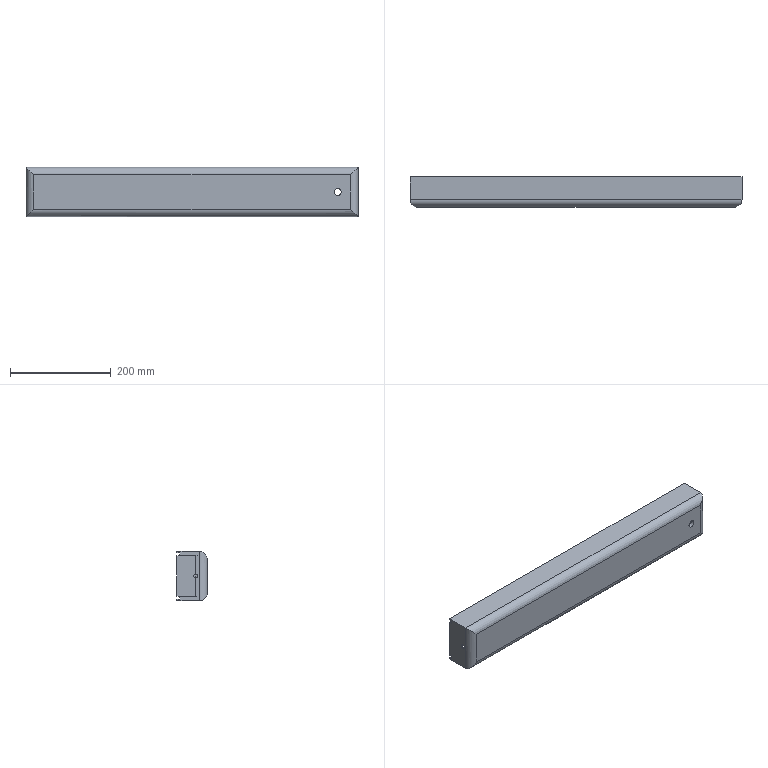Part | SolidWorks | features BaseBody 1 | 1 solid | 34 faces | box 660 x 60.3 x 97.82 mm | volume 1057763 mm3 | plane 22 | cylinder 12 | commonest cylinder face diameters 30 x8 8 x2 14 x2
STEP:
#1=CARTESIAN_POINT('',(-747.81,92.16,59.05));
#2=VERTEX_POINT('',#1);
#3=CARTESIAN_POINT('',(-750.,92.16,59.05));
#4=VERTEX_POINT('',#3);
#5=CARTESIAN_POINT('',(-747.81,92.16,59.05));
#6=DIRECTION('',(-1.,0.,0.));
#7=VECTOR('',#6,1000.);
#8=LINE('',#5,#7);
#9=EDGE_CURVE('',#2,#4,#8,.T.);
#10=ORIENTED_EDGE('',*,*,#9,.F.);
#11=CARTESIAN_POINT('',(-747.81,92.16,-21.25));
#12=VERTEX_POINT('',#11);
#13=CARTESIAN_POINT('',(-747.81,92.16,-21.25));
#14=DIRECTION('',(0.,0.,1.));
#15=VECTOR('',#14,1000.);
#16=LINE('',#13,#15);
#17=EDGE_CURVE('',#12,#2,#16,.T.);
#18=ORIENTED_EDGE('',*,*,#17,.F.);
#19=CARTESIAN_POINT('',(-750.,92.16,-21.25));
#20=VERTEX_POINT('',#19);
#21=CARTESIAN_POINT('',(-750.,92.16,-21.25));
#22=DIRECTION('',(1.,0.,0.));
#23=VECTOR('',#22,1000.);
#24=LINE('',#21,#23);
#25=EDGE_CURVE('',#20,#12,#24,.T.);
#26=ORIENTED_EDGE('',*,*,#25,.F.);
#27=CARTESIAN_POINT('',(-750.,92.16,59.05));
#28=DIRECTION('',(0.,0.,-1.));
#29=VECTOR('',#28,1000.);
#30=LINE('',#27,#29);
#31=EDGE_CURVE('',#4,#20,#30,.T.);
#32=ORIENTED_EDGE('',*,*,#31,.F.);
#33=EDGE_LOOP('',(#10,#18,#26,#32));
#34=FACE_OUTER_BOUND('',#33,.T.);
#35=CARTESIAN_POINT('',(-1290.2,92.16,18.9));
#36=DIRECTION('',(0.,1.,0.));
#37=DIRECTION('',(1.,0.,0.));
#38=AXIS2_PLACEMENT_3D('',#35,#36,#37);
#39=PLANE('',#38);
#40=ADVANCED_FACE('',(#34),#39,.T.);
#41=CARTESIAN_POINT('',(-750.,86.32,-21.25));
#42=VERTEX_POINT('',#41);
#43=CARTESIAN_POINT('',(-747.81,86.32,-21.25));
#44=VERTEX_POINT('',#43);
#45=CARTESIAN_POINT('',(-750.,86.32,-21.25));
#46=DIRECTION('',(1.,0.,0.));
#47=VECTOR('',#46,1000.);
#48=LINE('',#45,#47);
#49=EDGE_CURVE('',#42,#44,#48,.T.);
#50=ORIENTED_EDGE('',*,*,#49,.F.);
#51=CARTESIAN_POINT('',(-750.,92.16,-21.25));
#52=DIRECTION('',(0.,-1.,0.));
#53=VECTOR('',#52,1000.);
#54=LINE('',#51,#53);
#55=EDGE_CURVE('',#20,#42,#54,.T.);
#56=ORIENTED_EDGE('',*,*,#55,.F.);
#57=ORIENTED_EDGE('',*,*,#25,.T.);
#58=CARTESIAN_POINT('',(-747.81,86.32,-21.25));
#59=DIRECTION('',(0.,1.,0.));
#60=VECTOR('',#59,1000.);
#61=LINE('',#58,#60);
#62=EDGE_CURVE('',#44,#12,#61,.T.);
#63=ORIENTED_EDGE('',*,*,#62,.F.);
#64=EDGE_LOOP('',(#50,#56,#57,#63));
#65=FACE_OUTER_BOUND('',#64,.T.);
#66=CARTESIAN_POINT('',(-750.,92.16,-21.25));
#67=DIRECTION('',(0.,0.,-1.));
#68=DIRECTION('',(0.,-1.,0.));
#69=AXIS2_PLACEMENT_3D('',#66,#67,#68);
#70=PLANE('',#69);
#71=ADVANCED_FACE('',(#65),#70,.T.);
#72=CARTESIAN_POINT('',(-747.81,86.32,59.05));
#73=VERTEX_POINT('',#72);
#74=CARTESIAN_POINT('',(-750.,86.32,59.05));
#75=VERTEX_POINT('',#74);
#76=CARTESIAN_POINT('',(-747.81,86.32,59.05));
#77=DIRECTION('',(-1.,0.,0.));
#78=VECTOR('',#77,1000.);
#79=LINE('',#76,#78);
#80=EDGE_CURVE('',#73,#75,#79,.T.);
#81=ORIENTED_EDGE('',*,*,#80,.F.);
#82=CARTESIAN_POINT('',(-747.81,92.16,59.05));
#83=DIRECTION('',(0.,-1.,0.));
#84=VECTOR('',#83,1000.);
#85=LINE('',#82,#84);
#86=EDGE_CURVE('',#2,#73,#85,.T.);
#87=ORIENTED_EDGE('',*,*,#86,.F.);
#88=ORIENTED_EDGE('',*,*,#9,.T.);
#89=CARTESIAN_POINT('',(-750.,86.32,59.05));
#90=DIRECTION('',(0.,1.,0.));
#91=VECTOR('',#90,1000.);
#92=LINE('',#89,#91);
#93=EDGE_CURVE('',#75,#4,#92,.T.);
#94=ORIENTED_EDGE('',*,*,#93,.F.);
#95=EDGE_LOOP('',(#81,#87,#88,#94));
#96=FACE_OUTER_BOUND('',#95,.T.);
#97=CARTESIAN_POINT('',(-750.,92.16,59.05));
#98=DIRECTION('',(0.,0.,1.));
#99=DIRECTION('',(1.,0.,0.));
#100=AXIS2_PLACEMENT_3D('',#97,#98,#99);
#101=PLANE('',#100);
#102=ADVANCED_FACE('',(#96),#101,.T.);
#103=CARTESIAN_POINT('',(-750.,92.16,-30.01));
#104=VERTEX_POINT('',#103);
#105=CARTESIAN_POINT('',(-90.,92.16,-30.01));
#106=VERTEX_POINT('',#105);
#107=CARTESIAN_POINT('',(-750.,92.16,-30.01));
#108=DIRECTION('',(1.,0.,0.));
#109=VECTOR('',#108,1000.);
#110=LINE('',#107,#109);
#111=EDGE_CURVE('',#104,#106,#110,.T.);
#112=ORIENTED_EDGE('',*,*,#111,.F.);
#113=CARTESIAN_POINT('',(-750.,92.16,-27.09));
#114=VERTEX_POINT('',#113);
#115=CARTESIAN_POINT('',(-750.,92.16,-27.09));
#116=DIRECTION('',(0.,0.,-1.));
#117=VECTOR('',#116,1000.);
#118=LINE('',#115,#117);
#119=EDGE_CURVE('',#114,#104,#118,.T.);
#120=ORIENTED_EDGE('',*,*,#119,.F.);
#121=CARTESIAN_POINT('',(-90.,92.16,-27.09));
#122=VERTEX_POINT('',#121);
#123=CARTESIAN_POINT('',(-90.,92.16,-27.09));
#124=DIRECTION('',(-1.,0.,0.));
#125=VECTOR('',#124,1000.);
#126=LINE('',#123,#125);
#127=EDGE_CURVE('',#122,#114,#126,.T.);
#128=ORIENTED_EDGE('',*,*,#127,.F.);
#129=CARTESIAN_POINT('',(-90.,92.16,-30.01));
#130=DIRECTION('',(0.,0.,1.));
#131=VECTOR('',#130,1000.);
#132=LINE('',#129,#131);
#133=EDGE_CURVE('',#106,#122,#132,.T.);
#134=ORIENTED_EDGE('',*,*,#133,.F.);
#135=EDGE_LOOP('',(#112,#120,#128,#134));
#136=FACE_OUTER_BOUND('',#135,.T.);
#137=CARTESIAN_POINT('',(-202.5,92.16,18.9));
#138=DIRECTION('',(0.,1.,0.));
#139=DIRECTION('',(1.,0.,0.));
#140=AXIS2_PLACEMENT_3D('',#137,#138,#139);
#141=PLANE('',#140);
#142=ADVANCED_FACE('',(#136),#141,.T.);
#143=ORIENTED_EDGE('',*,*,#127,.T.);
#144=CARTESIAN_POINT('',(-750.,86.32,-27.09));
#145=VERTEX_POINT('',#144);
#146=CARTESIAN_POINT('',(-750.,86.32,-27.09));
#147=DIRECTION('',(0.,1.,0.));
#148=VECTOR('',#147,1000.);
#149=LINE('',#146,#148);
#150=EDGE_CURVE('',#145,#114,#149,.T.);
#151=ORIENTED_EDGE('',*,*,#150,.F.);
#152=CARTESIAN_POINT('',(-90.,86.32,-27.09));
#153=VERTEX_POINT('',#152);
#154=CARTESIAN_POINT('',(-90.,86.32,-27.09));
#155=DIRECTION('',(-1.,0.,0.));
#156=VECTOR('',#155,1000.);
#157=LINE('',#154,#156);
#158=EDGE_CURVE('',#153,#145,#157,.T.);
#159=ORIENTED_EDGE('',*,*,#158,.F.);
#160=CARTESIAN_POINT('',(-90.,92.16,-27.09));
#161=DIRECTION('',(0.,-1.,0.));
#162=VECTOR('',#161,1000.);
#163=LINE('',#160,#162);
#164=EDGE_CURVE('',#122,#153,#163,.T.);
#165=ORIENTED_EDGE('',*,*,#164,.F.);
#166=EDGE_LOOP('',(#143,#151,#159,#165));
#167=FACE_OUTER_BOUND('',#166,.T.);
#168=CARTESIAN_POINT('',(-750.,92.16,-27.09));
#169=DIRECTION('',(0.,0.,1.));
#170=DIRECTION('',(1.,0.,0.));
#171=AXIS2_PLACEMENT_3D('',#168,#169,#170);
#172=PLANE('',#171);
#173=ADVANCED_FACE('',(#167),#172,.T.);
#174=ORIENTED_EDGE('',*,*,#158,.T.);
#175=CARTESIAN_POINT('',(-750.,86.32,-21.25));
#176=DIRECTION('',(0.,0.,-1.));
#177=VECTOR('',#176,1000.);
#178=LINE('',#175,#177);
#179=EDGE_CURVE('',#42,#145,#178,.T.);
#180=ORIENTED_EDGE('',*,*,#179,.F.);
#181=ORIENTED_EDGE('',*,*,#49,.T.);
#182=CARTESIAN_POINT('',(-93.,86.32,-21.25));
#183=VERTEX_POINT('',#182);
#184=CARTESIAN_POINT('',(-93.,86.32,-21.25));
#185=DIRECTION('',(-1.,0.,0.));
#186=VECTOR('',#185,1000.);
#187=LINE('',#184,#186);
#188=EDGE_CURVE('',#183,#44,#187,.T.);
#189=ORIENTED_EDGE('',*,*,#188,.F.);
#190=CARTESIAN_POINT('',(-90.,86.32,-21.25));
#191=VERTEX_POINT('',#190);
#192=CARTESIAN_POINT('',(-90.,86.32,-21.25));
#193=DIRECTION('',(-1.,0.,0.));
#194=VECTOR('',#193,1000.);
#195=LINE('',#192,#194);
#196=EDGE_CURVE('',#191,#183,#195,.T.);
#197=ORIENTED_EDGE('',*,*,#196,.F.);
#198=CARTESIAN_POINT('',(-90.,86.32,-27.09));
#199=DIRECTION('',(0.,0.,1.));
#200=VECTOR('',#199,1000.);
#201=LINE('',#198,#200);
#202=EDGE_CURVE('',#153,#191,#201,.T.);
#203=ORIENTED_EDGE('',*,*,#202,.F.);
#204=EDGE_LOOP('',(#174,#180,#181,#189,#197,#203));
#205=FACE_OUTER_BOUND('',#204,.T.);
#206=CARTESIAN_POINT('',(-750.,86.32,64.89));
#207=DIRECTION('',(0.,1.,0.));
#208=DIRECTION('',(1.,0.,0.));
#209=AXIS2_PLACEMENT_3D('',#206,#207,#208);
#210=PLANE('',#209);
#211=ADVANCED_FACE('',(#205),#210,.T.);
#212=CARTESIAN_POINT('',(-747.81,54.16,-21.25));
#213=VERTEX_POINT('',#212);
#214=CARTESIAN_POINT('',(-747.81,54.16,-21.25));
#215=DIRECTION('',(0.,1.,0.));
#216=VECTOR('',#215,1000.);
#217=LINE('',#214,#216);
#218=EDGE_CURVE('',#213,#44,#217,.T.);
#219=ORIENTED_EDGE('',*,*,#218,.F.);
#220=CARTESIAN_POINT('',(-93.,54.16,-21.25));
#221=VERTEX_POINT('',#220);
#222=CARTESIAN_POINT('',(-93.,54.16,-21.25));
#223=DIRECTION('',(-1.,0.,0.));
#224=VECTOR('',#223,1000.);
#225=LINE('',#222,#224);
#226=EDGE_CURVE('',#221,#213,#225,.T.);
#227=ORIENTED_EDGE('',*,*,#226,.F.);
#228=CARTESIAN_POINT('',(-93.,86.32,-21.25));
#229=DIRECTION('',(0.,-1.,0.));
#230=VECTOR('',#229,1000.);
#231=LINE('',#228,#230);
#232=EDGE_CURVE('',#183,#221,#231,.T.);
#233=ORIENTED_EDGE('',*,*,#232,.F.);
#234=ORIENTED_EDGE('',*,*,#188,.T.);
#235=EDGE_LOOP('',(#219,#227,#233,#234));
#236=FACE_OUTER_BOUND('',#235,.T.);
#237=CARTESIAN_POINT('',(-742.7,19.16,-21.25));
#238=DIRECTION('',(0.,0.,1.));
#239=DIRECTION('',(1.,0.,0.));
#240=AXIS2_PLACEMENT_3D('',#237,#238,#239);
#241=PLANE('',#240);
#242=ADVANCED_FACE('',(#236),#241,.T.);
#243=CARTESIAN_POINT('',(-93.,86.32,59.05));
#244=VERTEX_POINT('',#243);
#245=CARTESIAN_POINT('',(-747.81,86.32,59.05));
#246=DIRECTION('',(1.,0.,0.));
#247=VECTOR('',#246,1000.);
#248=LINE('',#245,#247);
#249=EDGE_CURVE('',#73,#244,#248,.T.);
#250=ORIENTED_EDGE('',*,*,#249,.F.);
#251=ORIENTED_EDGE('',*,*,#80,.T.);
#252=CARTESIAN_POINT('',(-750.,86.32,64.89));
#253=VERTEX_POINT('',#252);
#254=CARTESIAN_POINT('',(-750.,86.32,64.89));
#255=DIRECTION('',(0.,0.,-1.));
#256=VECTOR('',#255,1000.);
#257=LINE('',#254,#256);
#258=EDGE_CURVE('',#253,#75,#257,.T.);
#259=ORIENTED_EDGE('',*,*,#258,.F.);
#260=CARTESIAN_POINT('',(-90.,86.32,64.89));
#261=VERTEX_POINT('',#260);
#262=CARTESIAN_POINT('',(-90.,86.32,64.89));
#263=DIRECTION('',(-1.,0.,0.));
#264=VECTOR('',#263,1000.);
#265=LINE('',#262,#264);
#266=EDGE_CURVE('',#261,#253,#265,.T.);
#267=ORIENTED_EDGE('',*,*,#266,.F.);
#268=CARTESIAN_POINT('',(-90.,86.32,59.05));
#269=VERTEX_POINT('',#268);
#270=CARTESIAN_POINT('',(-90.,86.32,59.05));
#271=DIRECTION('',(0.,0.,1.));
#272=VECTOR('',#271,1000.);
#273=LINE('',#270,#272);
#274=EDGE_CURVE('',#269,#261,#273,.T.);
#275=ORIENTED_EDGE('',*,*,#274,.F.);
#276=CARTESIAN_POINT('',(-93.,86.32,59.05));
#277=DIRECTION('',(1.,0.,0.));
#278=VECTOR('',#277,1000.);
#279=LINE('',#276,#278);
#280=EDGE_CURVE('',#244,#269,#279,.T.);
#281=ORIENTED_EDGE('',*,*,#280,.F.);
#282=EDGE_LOOP('',(#250,#251,#259,#267,#275,#281));
#283=FACE_OUTER_BOUND('',#282,.T.);
#284=CARTESIAN_POINT('',(-750.,86.32,64.89));
#285=DIRECTION('',(0.,1.,0.));
#286=DIRECTION('',(1.,0.,0.));
#287=AXIS2_PLACEMENT_3D('',#284,#285,#286);
#288=PLANE('',#287);
#289=ADVANCED_FACE('',(#283),#288,.T.);
#290=ORIENTED_EDGE('',*,*,#266,.T.);
#291=CARTESIAN_POINT('',(-750.,92.16,64.89));
#292=VERTEX_POINT('',#291);
#293=CARTESIAN_POINT('',(-750.,92.16,64.89));
#294=DIRECTION('',(0.,-1.,0.));
#295=VECTOR('',#294,1000.);
#296=LINE('',#293,#295);
#297=EDGE_CURVE('',#292,#253,#296,.T.);
#298=ORIENTED_EDGE('',*,*,#297,.F.);
#299=CARTESIAN_POINT('',(-90.,92.16,64.89));
#300=VERTEX_POINT('',#299);
#301=CARTESIAN_POINT('',(-90.,92.16,64.89));
#302=DIRECTION('',(-1.,0.,0.));
#303=VECTOR('',#302,1000.);
#304=LINE('',#301,#303);
#305=EDGE_CURVE('',#300,#292,#304,.T.);
#306=ORIENTED_EDGE('',*,*,#305,.F.);
#307=CARTESIAN_POINT('',(-90.,86.32,64.89));
#308=DIRECTION('',(0.,1.,0.));
#309=VECTOR('',#308,1000.);
#310=LINE('',#307,#309);
#311=EDGE_CURVE('',#261,#300,#310,.T.);
#312=ORIENTED_EDGE('',*,*,#311,.F.);
#313=EDGE_LOOP('',(#290,#298,#306,#312));
#314=FACE_OUTER_BOUND('',#313,.T.);
#315=CARTESIAN_POINT('',(-750.,92.16,64.89));
#316=DIRECTION('',(0.,0.,-1.));
#317=DIRECTION('',(0.,-1.,0.));
#318=AXIS2_PLACEMENT_3D('',#315,#316,#317);
#319=PLANE('',#318);
#320=ADVANCED_FACE('',(#314),#319,.T.);
#321=ORIENTED_EDGE('',*,*,#305,.T.);
#322=CARTESIAN_POINT('',(-750.,92.16,67.81));
#323=VERTEX_POINT('',#322);
#324=CARTESIAN_POINT('',(-750.,92.16,67.81));
#325=DIRECTION('',(0.,0.,-1.));
#326=VECTOR('',#325,1000.);
#327=LINE('',#324,#326);
#328=EDGE_CURVE('',#323,#292,#327,.T.);
#329=ORIENTED_EDGE('',*,*,#328,.F.);
#330=CARTESIAN_POINT('',(-90.,92.16,67.81));
#331=VERTEX_POINT('',#330);
#332=CARTESIAN_POINT('',(-90.,92.16,67.81));
#333=DIRECTION('',(-1.,0.,0.));
#334=VECTOR('',#333,1000.);
#335=LINE('',#332,#334);
#336=EDGE_CURVE('',#331,#323,#335,.T.);
#337=ORIENTED_EDGE('',*,*,#336,.F.);
#338=CARTESIAN_POINT('',(-90.,92.16,64.89));
#339=DIRECTION('',(0.,0.,1.));
#340=VECTOR('',#339,1000.);
#341=LINE('',#338,#340);
#342=EDGE_CURVE('',#300,#331,#341,.T.);
#343=ORIENTED_EDGE('',*,*,#342,.F.);
#344=EDGE_LOOP('',(#321,#329,#337,#343));
#345=FACE_OUTER_BOUND('',#344,.T.);
#346=CARTESIAN_POINT('',(-202.5,92.16,18.9));
#347=DIRECTION('',(0.,1.,0.));
#348=DIRECTION('',(1.,0.,0.));
#349=AXIS2_PLACEMENT_3D('',#346,#347,#348);
#350=PLANE('',#349);
#351=ADVANCED_FACE('',(#345),#350,.T.);
#352=CARTESIAN_POINT('',(-90.,92.16,59.05));
#353=VERTEX_POINT('',#352);
#354=CARTESIAN_POINT('',(-90.,92.16,59.05));
#355=DIRECTION('',(0.,-1.,0.));
#356=VECTOR('',#355,1000.);
#357=LINE('',#354,#356);
#358=EDGE_CURVE('',#353,#269,#357,.T.);
#359=ORIENTED_EDGE('',*,*,#358,.F.);
#360=CARTESIAN_POINT('',(-93.,92.16,59.05));
#361=VERTEX_POINT('',#360);
#362=CARTESIAN_POINT('',(-93.,92.16,59.05));
#363=DIRECTION('',(1.,0.,0.));
#364=VECTOR('',#363,1000.);
#365=LINE('',#362,#364);
#366=EDGE_CURVE('',#361,#353,#365,.T.);
#367=ORIENTED_EDGE('',*,*,#366,.F.);
#368=CARTESIAN_POINT('',(-93.,86.32,59.05));
#369=DIRECTION('',(0.,1.,0.));
#370=VECTOR('',#369,1000.);
#371=LINE('',#368,#370);
#372=EDGE_CURVE('',#244,#361,#371,.T.);
#373=ORIENTED_EDGE('',*,*,#372,.F.);
#374=ORIENTED_EDGE('',*,*,#280,.T.);
#375=EDGE_LOOP('',(#359,#367,#373,#374));
#376=FACE_OUTER_BOUND('',#375,.T.);
#377=CARTESIAN_POINT('',(-90.,86.32,59.05));
#378=DIRECTION('',(0.,0.,1.));
#379=DIRECTION('',(0.,-1.,0.));
#380=AXIS2_PLACEMENT_3D('',#377,#378,#379);
#381=PLANE('',#380);
#382=ADVANCED_FACE('',(#376),#381,.T.);
#383=CARTESIAN_POINT('',(-90.,92.16,-21.25));
#384=VERTEX_POINT('',#383);
#385=CARTESIAN_POINT('',(-90.,92.16,-21.25));
#386=DIRECTION('',(0.,0.,1.));
#387=VECTOR('',#386,1000.);
#388=LINE('',#385,#387);
#389=EDGE_CURVE('',#384,#353,#388,.T.);
#390=ORIENTED_EDGE('',*,*,#389,.F.);
#391=CARTESIAN_POINT('',(-93.,92.16,-21.25));
#392=VERTEX_POINT('',#391);
#393=CARTESIAN_POINT('',(-93.,92.16,-21.25));
#394=DIRECTION('',(1.,0.,0.));
#395=VECTOR('',#394,1000.);
#396=LINE('',#393,#395);
#397=EDGE_CURVE('',#392,#384,#396,.T.);
#398=ORIENTED_EDGE('',*,*,#397,.F.);
#399=CARTESIAN_POINT('',(-93.,92.16,59.05));
#400=DIRECTION('',(0.,0.,-1.));
#401=VECTOR('',#400,1000.);
#402=LINE('',#399,#401);
#403=EDGE_CURVE('',#361,#392,#402,.T.);
#404=ORIENTED_EDGE('',*,*,#403,.F.);
#405=ORIENTED_EDGE('',*,*,#366,.T.);
#406=EDGE_LOOP('',(#390,#398,#404,#405));
#407=FACE_OUTER_BOUND('',#406,.T.);
#408=CARTESIAN_POINT('',(-90.,92.16,59.05));
#409=DIRECTION('',(0.,1.,0.));
#410=DIRECTION('',(1.,0.,0.));
#411=AXIS2_PLACEMENT_3D('',#408,#409,#410);
#412=PLANE('',#411);
#413=ADVANCED_FACE('',(#407),#412,.T.);
#414=CARTESIAN_POINT('',(-90.,86.32,-21.25));
#415=DIRECTION('',(0.,1.,0.));
#416=VECTOR('',#415,1000.);
#417=LINE('',#414,#416);
#418=EDGE_CURVE('',#191,#384,#417,.T.);
#419=ORIENTED_EDGE('',*,*,#418,.F.);
#420=ORIENTED_EDGE('',*,*,#196,.T.);
#421=CARTESIAN_POINT('',(-93.,92.16,-21.25));
#422=DIRECTION('',(0.,-1.,0.));
#423=VECTOR('',#422,1000.);
#424=LINE('',#421,#423);
#425=EDGE_CURVE('',#392,#183,#424,.T.);
#426=ORIENTED_EDGE('',*,*,#425,.F.);
#427=ORIENTED_EDGE('',*,*,#397,.T.);
#428=EDGE_LOOP('',(#419,#420,#426,#427));
#429=FACE_OUTER_BOUND('',#428,.T.);
#430=CARTESIAN_POINT('',(-90.,92.16,-21.25));
#431=DIRECTION('',(0.,0.,-1.));
#432=DIRECTION('',(0.,-1.,0.));
#433=AXIS2_PLACEMENT_3D('',#430,#431,#432);
#434=PLANE('',#433);
#435=ADVANCED_FACE('',(#429),#434,.T.);
#436=CARTESIAN_POINT('',(-750.,54.36,22.9));
#437=VERTEX_POINT('',#436);
#438=CARTESIAN_POINT('',(-750.,54.36,14.9));
#439=VERTEX_POINT('',#438);
#440=CARTESIAN_POINT('',(-750.,54.36,18.9));
#441=DIRECTION('',(-1.,0.,0.));
#442=DIRECTION('',(0.,0.,1.));
#443=AXIS2_PLACEMENT_3D('',#440,#441,#442);
#444=CIRCLE('',#443,4.);
#445=EDGE_CURVE('',#437,#439,#444,.T.);
#446=ORIENTED_EDGE('',*,*,#445,.F.);
#447=CARTESIAN_POINT('',(-750.,54.36,18.9));
#448=DIRECTION('',(-1.,0.,0.));
#449=DIRECTION('',(0.,0.,-1.));
#450=AXIS2_PLACEMENT_3D('',#447,#448,#449);
#451=CIRCLE('',#450,4.);
#452=EDGE_CURVE('',#439,#437,#451,.T.);
#453=ORIENTED_EDGE('',*,*,#452,.F.);
#454=EDGE_LOOP('',(#446,#453));
#455=FACE_BOUND('',#454,.T.);
#456=CARTESIAN_POINT('',(-750.,46.86,67.81));
#457=VERTEX_POINT('',#456);
#458=CARTESIAN_POINT('',(-750.,92.16,67.81));
#459=DIRECTION('',(0.,-1.,0.));
#460=VECTOR('',#459,1000.);
#461=LINE('',#458,#460);
#462=EDGE_CURVE('',#323,#457,#461,.T.);
#463=ORIENTED_EDGE('',*,*,#462,.F.);
#464=ORIENTED_EDGE('',*,*,#328,.T.);
#465=ORIENTED_EDGE('',*,*,#297,.T.);
#466=ORIENTED_EDGE('',*,*,#258,.T.);
#467=ORIENTED_EDGE('',*,*,#93,.T.);
#468=ORIENTED_EDGE('',*,*,#31,.T.);
#469=ORIENTED_EDGE('',*,*,#55,.T.);
#470=ORIENTED_EDGE('',*,*,#179,.T.);
#471=ORIENTED_EDGE('',*,*,#150,.T.);
#472=ORIENTED_EDGE('',*,*,#119,.T.);
#473=CARTESIAN_POINT('',(-750.,46.86,-30.01));
#474=VERTEX_POINT('',#473);
#475=CARTESIAN_POINT('',(-750.,46.86,-30.01));
#476=DIRECTION('',(0.,1.,0.));
#477=VECTOR('',#476,1000.);
#478=LINE('',#475,#477);
#479=EDGE_CURVE('',#474,#104,#478,.T.);
#480=ORIENTED_EDGE('',*,*,#479,.F.);
#481=CARTESIAN_POINT('',(-750.,46.86,67.81));
#482=DIRECTION('',(0.,0.,-1.));
#483=VECTOR('',#482,1000.);
#484=LINE('',#481,#483);
#485=EDGE_CURVE('',#457,#474,#484,.T.);
#486=ORIENTED_EDGE('',*,*,#485,.F.);
#487=EDGE_LOOP('',(#463,#464,#465,#466,#467,#468,#469,#470,#471,#472,#480,#486));
#488=FACE_OUTER_BOUND('',#487,.T.);
#489=CARTESIAN_POINT('',(-750.,46.17,18.9));
#490=DIRECTION('',(-1.,0.,0.));
#491=DIRECTION('',(0.,0.,1.));
#492=AXIS2_PLACEMENT_3D('',#489,#490,#491);
#493=PLANE('',#492);
#494=ADVANCED_FACE('',(#455,#488),#493,.T.);
#495=CARTESIAN_POINT('',(-90.,46.86,-30.01));
#496=VERTEX_POINT('',#495);
#497=CARTESIAN_POINT('',(-90.,46.86,-30.01));
#498=DIRECTION('',(0.,1.,0.));
#499=VECTOR('',#498,1000.);
#500=LINE('',#497,#499);
#501=EDGE_CURVE('',#496,#106,#500,.T.);
#502=ORIENTED_EDGE('',*,*,#501,.F.);
#503=CARTESIAN_POINT('',(-750.,46.86,-30.01));
#504=DIRECTION('',(1.,0.,0.));
#505=VECTOR('',#504,1000.);
#506=LINE('',#503,#505);
#507=EDGE_CURVE('',#474,#496,#506,.T.);
#508=ORIENTED_EDGE('',*,*,#507,.F.);
#509=ORIENTED_EDGE('',*,*,#479,.T.);
#510=ORIENTED_EDGE('',*,*,#111,.T.);
#511=EDGE_LOOP('',(#502,#508,#509,#510));
#512=FACE_OUTER_BOUND('',#511,.T.);
#513=CARTESIAN_POINT('',(-750.,92.16,-30.01));
#514=DIRECTION('',(0.,0.,-1.));
#515=DIRECTION('',(0.,-1.,0.));
#516=AXIS2_PLACEMENT_3D('',#513,#514,#515);
#517=PLANE('',#516);
#518=ADVANCED_FACE('',(#512),#517,.T.);
#519=CARTESIAN_POINT('',(-90.,46.86,67.81));
#520=VERTEX_POINT('',#519);
#521=CARTESIAN_POINT('',(-90.,46.86,67.81));
#522=DIRECTION('',(0.,1.,0.));
#523=VECTOR('',#522,1000.);
#524=LINE('',#521,#523);
#525=EDGE_CURVE('',#520,#331,#524,.T.);
#526=ORIENTED_EDGE('',*,*,#525,.F.);
#527=CARTESIAN_POINT('',(-90.,46.86,-30.01));
#528=DIRECTION('',(0.,0.,1.));
#529=VECTOR('',#528,1000.);
#530=LINE('',#527,#529);
#531=EDGE_CURVE('',#496,#520,#530,.T.);
#532=ORIENTED_EDGE('',*,*,#531,.F.);
#533=ORIENTED_EDGE('',*,*,#501,.T.);
#534=ORIENTED_EDGE('',*,*,#133,.T.);
#535=ORIENTED_EDGE('',*,*,#164,.T.);
#536=ORIENTED_EDGE('',*,*,#202,.T.);
#537=ORIENTED_EDGE('',*,*,#418,.T.);
#538=ORIENTED_EDGE('',*,*,#389,.T.);
#539=ORIENTED_EDGE('',*,*,#358,.T.);
#540=ORIENTED_EDGE('',*,*,#274,.T.);
#541=ORIENTED_EDGE('',*,*,#311,.T.);
#542=ORIENTED_EDGE('',*,*,#342,.T.);
#543=EDGE_LOOP('',(#526,#532,#533,#534,#535,#536,#537,#538,#539,#540,#541,#542));
#544=FACE_OUTER_BOUND('',#543,.T.);
#545=CARTESIAN_POINT('',(-90.,52.01,18.9));
#546=DIRECTION('',(1.,0.,0.));
#547=DIRECTION('',(0.,1.,0.));
#548=AXIS2_PLACEMENT_3D('',#545,#546,#547);
#549=PLANE('',#548);
#550=ADVANCED_FACE('',(#544),#549,.T.);
#551=CARTESIAN_POINT('',(-747.81,54.16,59.05));
#552=VERTEX_POINT('',#551);
#553=CARTESIAN_POINT('',(-747.81,86.32,59.05));
#554=DIRECTION('',(0.,-1.,0.));
#555=VECTOR('',#554,1000.);
#556=LINE('',#553,#555);
#557=EDGE_CURVE('',#73,#552,#556,.T.);
#558=ORIENTED_EDGE('',*,*,#557,.F.);
#559=ORIENTED_EDGE('',*,*,#249,.T.);
#560=CARTESIAN_POINT('',(-93.,54.16,59.05));
#561=VERTEX_POINT('',#560);
#562=CARTESIAN_POINT('',(-93.,54.16,59.05));
#563=DIRECTION('',(0.,1.,0.));
#564=VECTOR('',#563,1000.);
#565=LINE('',#562,#564);
#566=EDGE_CURVE('',#561,#244,#565,.T.);
#567=ORIENTED_EDGE('',*,*,#566,.F.);
#568=CARTESIAN_POINT('',(-747.81,54.16,59.05));
#569=DIRECTION('',(1.,0.,0.));
#570=VECTOR('',#569,1000.);
#571=LINE('',#568,#570);
#572=EDGE_CURVE('',#552,#561,#571,.T.);
#573=ORIENTED_EDGE('',*,*,#572,.F.);
#574=EDGE_LOOP('',(#558,#559,#567,#573));
#575=FACE_OUTER_BOUND('',#574,.T.);
#576=CARTESIAN_POINT('',(-742.7,19.16,59.05));
#577=DIRECTION('',(0.,0.,-1.));
#578=DIRECTION('',(0.,-1.,0.));
#579=AXIS2_PLACEMENT_3D('',#576,#577,#578);
#580=PLANE('',#579);
#581=ADVANCED_FACE('',(#575),#580,.T.);
#582=ORIENTED_EDGE('',*,*,#566,.T.);
#583=ORIENTED_EDGE('',*,*,#372,.T.);
#584=ORIENTED_EDGE('',*,*,#403,.T.);
#585=ORIENTED_EDGE('',*,*,#425,.T.);
#586=ORIENTED_EDGE('',*,*,#232,.T.);
#587=CARTESIAN_POINT('',(-93.,54.16,59.05));
#588=DIRECTION('',(0.,0.,-1.));
#589=VECTOR('',#588,1000.);
#590=LINE('',#587,#589);
#591=EDGE_CURVE('',#561,#221,#590,.T.);
#592=ORIENTED_EDGE('',*,*,#591,.F.);
#593=EDGE_LOOP('',(#582,#583,#584,#585,#586,#592));
#594=FACE_OUTER_BOUND('',#593,.T.);
#595=CARTESIAN_POINT('',(-93.,52.01,18.9));
#596=DIRECTION('',(-1.,0.,0.));
#597=DIRECTION('',(0.,0.,1.));
#598=AXIS2_PLACEMENT_3D('',#595,#596,#597);
#599=PLANE('',#598);
#600=ADVANCED_FACE('',(#594),#599,.T.);
#601=CARTESIAN_POINT('',(-123.,31.86,18.9));
#602=VERTEX_POINT('',#601);
#603=CARTESIAN_POINT('',(-137.,31.86,18.9));
#604=VERTEX_POINT('',#603);
#605=CARTESIAN_POINT('',(-130.,31.86,18.9));
#606=DIRECTION('',(0.,-1.,0.));
#607=DIRECTION('',(1.,0.,0.));
#608=AXIS2_PLACEMENT_3D('',#605,#606,#607);
#609=CIRCLE('',#608,7.);
#610=EDGE_CURVE('',#602,#604,#609,.T.);
#611=ORIENTED_EDGE('',*,*,#610,.F.);
#612=CARTESIAN_POINT('',(-130.,31.86,18.9));
#613=DIRECTION('',(0.,-1.,0.));
#614=DIRECTION('',(-1.,0.,0.));
#615=AXIS2_PLACEMENT_3D('',#612,#613,#614);
#616=CIRCLE('',#615,7.);
#617=EDGE_CURVE('',#604,#602,#616,.T.);
#618=ORIENTED_EDGE('',*,*,#617,.F.);
#619=EDGE_LOOP('',(#611,#618));
#620=FACE_BOUND('',#619,.T.);
#621=CARTESIAN_POINT('',(-735.,31.86,-15.01));
#622=VERTEX_POINT('',#621);
#623=CARTESIAN_POINT('',(-735.,31.86,52.81));
#624=VERTEX_POINT('',#623);
#625=CARTESIAN_POINT('',(-735.,31.86,-15.01));
#626=DIRECTION('',(0.,0.,1.));
#627=VECTOR('',#626,1000.);
#628=LINE('',#625,#627);
#629=EDGE_CURVE('',#622,#624,#628,.T.);
#630=ORIENTED_EDGE('',*,*,#629,.F.);
#631=CARTESIAN_POINT('',(-105.,31.86,-15.01));
#632=VERTEX_POINT('',#631);
#633=CARTESIAN_POINT('',(-105.,31.86,-15.01));
#634=DIRECTION('',(-1.,0.,0.));
#635=VECTOR('',#634,1000.);
#636=LINE('',#633,#635);
#637=EDGE_CURVE('',#632,#622,#636,.T.);
#638=ORIENTED_EDGE('',*,*,#637,.F.);
#639=CARTESIAN_POINT('',(-105.,31.86,52.81));
#640=VERTEX_POINT('',#639);
#641=CARTESIAN_POINT('',(-105.,31.86,52.81));
#642=DIRECTION('',(0.,0.,-1.));
#643=VECTOR('',#642,1000.);
#644=LINE('',#641,#643);
#645=EDGE_CURVE('',#640,#632,#644,.T.);
#646=ORIENTED_EDGE('',*,*,#645,.F.);
#647=CARTESIAN_POINT('',(-735.,31.86,52.81));
#648=DIRECTION('',(1.,0.,0.));
#649=VECTOR('',#648,1000.);
#650=LINE('',#647,#649);
#651=EDGE_CURVE('',#624,#640,#650,.T.);
#652=ORIENTED_EDGE('',*,*,#651,.F.);
#653=EDGE_LOOP('',(#630,#638,#646,#652));
#654=FACE_OUTER_BOUND('',#653,.T.);
#655=CARTESIAN_POINT('',(-202.5,31.86,18.9));
#656=DIRECTION('',(0.,-1.,0.));
#657=DIRECTION('',(0.,0.,-1.));
#658=AXIS2_PLACEMENT_3D('',#655,#656,#657);
#659=PLANE('',#658);
#660=ADVANCED_FACE('',(#620,#654),#659,.T.);
#661=ORIENTED_EDGE('',*,*,#507,.T.);
#662=CARTESIAN_POINT('',(-105.,31.86,-15.01));
#663=CARTESIAN_POINT('',(-96.213,31.86,-23.797));
#664=CARTESIAN_POINT('',(-90.,38.073,-30.01));
#665=CARTESIAN_POINT('',(-90.,46.86,-30.01));
#666=(BOUNDED_CURVE()B_SPLINE_CURVE(3,(#662,#663,#664,#665),.UNSPECIFIED.,.F.,.F.)B_SPLINE_CURVE_WITH_KNOTS((4,4),(4.712,6.283),.UNSPECIFIED.)CURVE()GEOMETRIC_REPRESENTATION_ITEM()RATIONAL_B_SPLINE_CURVE((1.,0.8047,0.8047,1.))REPRESENTATION_ITEM(''));
#667=EDGE_CURVE('',#632,#496,#666,.T.);
#668=ORIENTED_EDGE('',*,*,#667,.F.);
#669=ORIENTED_EDGE('',*,*,#637,.T.);
#670=CARTESIAN_POINT('',(-750.,46.86,-30.01));
#671=CARTESIAN_POINT('',(-750.,38.073,-30.01));
#672=CARTESIAN_POINT('',(-743.787,31.86,-23.797));
#673=CARTESIAN_POINT('',(-735.,31.86,-15.01));
#674=(BOUNDED_CURVE()B_SPLINE_CURVE(3,(#670,#671,#672,#673),.UNSPECIFIED.,.F.,.F.)B_SPLINE_CURVE_WITH_KNOTS((4,4),(0.,1.571),.UNSPECIFIED.)CURVE()GEOMETRIC_REPRESENTATION_ITEM()RATIONAL_B_SPLINE_CURVE((1.,0.8047,0.8047,1.))REPRESENTATION_ITEM(''));
#675=EDGE_CURVE('',#474,#622,#674,.T.);
#676=ORIENTED_EDGE('',*,*,#675,.F.);
#677=EDGE_LOOP('',(#661,#668,#669,#676));
#678=FACE_OUTER_BOUND('',#677,.T.);
#679=CARTESIAN_POINT('',(-90.,46.86,-15.01));
#680=DIRECTION('',(-1.,0.,0.));
#681=DIRECTION('',(0.,-1.,0.));
#682=AXIS2_PLACEMENT_3D('',#679,#680,#681);
#683=CYLINDRICAL_SURFACE('',#682,15.);
#684=ADVANCED_FACE('',(#678),#683,.T.);
#685=ORIENTED_EDGE('',*,*,#531,.T.);
#686=CARTESIAN_POINT('',(-105.,31.86,52.81));
#687=CARTESIAN_POINT('',(-96.213,31.86,61.597));
#688=CARTESIAN_POINT('',(-90.,38.073,67.81));
#689=CARTESIAN_POINT('',(-90.,46.86,67.81));
#690=(BOUNDED_CURVE()B_SPLINE_CURVE(3,(#686,#687,#688,#689),.UNSPECIFIED.,.F.,.T.)B_SPLINE_CURVE_WITH_KNOTS((4,4),(4.712,6.283),.UNSPECIFIED.)CURVE()GEOMETRIC_REPRESENTATION_ITEM()RATIONAL_B_SPLINE_CURVE((1.,0.8047,0.8047,1.))REPRESENTATION_ITEM(''));
#691=EDGE_CURVE('',#640,#520,#690,.T.);
#692=ORIENTED_EDGE('',*,*,#691,.F.);
#693=ORIENTED_EDGE('',*,*,#645,.T.);
#694=ORIENTED_EDGE('',*,*,#667,.T.);
#695=EDGE_LOOP('',(#685,#692,#693,#694));
#696=FACE_OUTER_BOUND('',#695,.T.);
#697=CARTESIAN_POINT('',(-105.,46.86,-30.01));
#698=DIRECTION('',(0.,0.,1.));
#699=DIRECTION('',(1.,0.000000424,0.));
#700=AXIS2_PLACEMENT_3D('',#697,#698,#699);
#701=CYLINDRICAL_SURFACE('',#700,15.);
#702=ADVANCED_FACE('',(#696),#701,.T.);
#703=CARTESIAN_POINT('',(-750.,46.86,67.81));
#704=DIRECTION('',(1.,0.,0.));
#705=VECTOR('',#704,1000.);
#706=LINE('',#703,#705);
#707=EDGE_CURVE('',#457,#520,#706,.T.);
#708=ORIENTED_EDGE('',*,*,#707,.F.);
#709=CARTESIAN_POINT('',(-735.,31.86,52.81));
#710=CARTESIAN_POINT('',(-743.787,31.86,61.597));
#711=CARTESIAN_POINT('',(-750.,38.073,67.81));
#712=CARTESIAN_POINT('',(-750.,46.86,67.81));
#713=(BOUNDED_CURVE()B_SPLINE_CURVE(3,(#709,#710,#711,#712),.UNSPECIFIED.,.F.,.F.)B_SPLINE_CURVE_WITH_KNOTS((4,4),(4.712,6.283),.UNSPECIFIED.)CURVE()GEOMETRIC_REPRESENTATION_ITEM()RATIONAL_B_SPLINE_CURVE((1.,0.8047,0.8047,1.))REPRESENTATION_ITEM(''));
#714=EDGE_CURVE('',#624,#457,#713,.T.);
#715=ORIENTED_EDGE('',*,*,#714,.F.);
#716=ORIENTED_EDGE('',*,*,#651,.T.);
#717=ORIENTED_EDGE('',*,*,#691,.T.);
#718=EDGE_LOOP('',(#708,#715,#716,#717));
#719=FACE_OUTER_BOUND('',#718,.T.);
#720=CARTESIAN_POINT('',(-750.,46.86,52.81));
#721=DIRECTION('',(1.,0.,0.));
#722=DIRECTION('',(0.,-1.,0.));
#723=AXIS2_PLACEMENT_3D('',#720,#721,#722);
#724=CYLINDRICAL_SURFACE('',#723,15.);
#725=ADVANCED_FACE('',(#719),#724,.T.);
#726=ORIENTED_EDGE('',*,*,#629,.T.);
#727=ORIENTED_EDGE('',*,*,#714,.T.);
#728=ORIENTED_EDGE('',*,*,#485,.T.);
#729=ORIENTED_EDGE('',*,*,#675,.T.);
#730=EDGE_LOOP('',(#726,#727,#728,#729));
#731=FACE_OUTER_BOUND('',#730,.T.);
#732=CARTESIAN_POINT('',(-735.,46.86,-30.01));
#733=DIRECTION('',(0.,0.,1.));
#734=DIRECTION('',(0.,-1.,0.));
#735=AXIS2_PLACEMENT_3D('',#732,#733,#734);
#736=CYLINDRICAL_SURFACE('',#735,15.);
#737=ADVANCED_FACE('',(#731),#736,.T.);
#738=CARTESIAN_POINT('',(-123.,39.16,18.9));
#739=VERTEX_POINT('',#738);
#740=CARTESIAN_POINT('',(-137.,39.16,18.9));
#741=VERTEX_POINT('',#740);
#742=CARTESIAN_POINT('',(-130.,39.16,18.9));
#743=DIRECTION('',(0.,1.,0.));
#744=DIRECTION('',(1.,0.,0.));
#745=AXIS2_PLACEMENT_3D('',#742,#743,#744);
#746=CIRCLE('',#745,7.);
#747=EDGE_CURVE('',#739,#741,#746,.T.);
#748=ORIENTED_EDGE('',*,*,#747,.F.);
#749=CARTESIAN_POINT('',(-130.,39.16,18.9));
#750=DIRECTION('',(0.,1.,0.));
#751=DIRECTION('',(-1.,0.,0.));
#752=AXIS2_PLACEMENT_3D('',#749,#750,#751);
#753=CIRCLE('',#752,7.);
#754=EDGE_CURVE('',#741,#739,#753,.T.);
#755=ORIENTED_EDGE('',*,*,#754,.F.);
#756=EDGE_LOOP('',(#748,#755));
#757=FACE_BOUND('',#756,.T.);
#758=CARTESIAN_POINT('',(-732.81,39.16,44.05));
#759=VERTEX_POINT('',#758);
#760=CARTESIAN_POINT('',(-732.81,39.16,-6.25));
#761=VERTEX_POINT('',#760);
#762=CARTESIAN_POINT('',(-732.81,39.16,44.05));
#763=DIRECTION('',(0.,0.,-1.));
#764=VECTOR('',#763,1000.);
#765=LINE('',#762,#764);
#766=EDGE_CURVE('',#759,#761,#765,.T.);
#767=ORIENTED_EDGE('',*,*,#766,.F.);
#768=CARTESIAN_POINT('',(-108.,39.16,44.05));
#769=VERTEX_POINT('',#768);
#770=CARTESIAN_POINT('',(-108.,39.16,44.05));
#771=DIRECTION('',(-1.,0.,0.));
#772=VECTOR('',#771,1000.);
#773=LINE('',#770,#772);
#774=EDGE_CURVE('',#769,#759,#773,.T.);
#775=ORIENTED_EDGE('',*,*,#774,.F.);
#776=CARTESIAN_POINT('',(-108.,39.16,-6.25));
#777=VERTEX_POINT('',#776);
#778=CARTESIAN_POINT('',(-108.,39.16,-6.25));
#779=DIRECTION('',(0.,0.,1.));
#780=VECTOR('',#779,1000.);
#781=LINE('',#778,#780);
#782=EDGE_CURVE('',#777,#769,#781,.T.);
#783=ORIENTED_EDGE('',*,*,#782,.F.);
#784=CARTESIAN_POINT('',(-732.81,39.16,-6.25));
#785=DIRECTION('',(1.,0.,0.));
#786=VECTOR('',#785,1000.);
#787=LINE('',#784,#786);
#788=EDGE_CURVE('',#761,#777,#787,.T.);
#789=ORIENTED_EDGE('',*,*,#788,.F.);
#790=EDGE_LOOP('',(#767,#775,#783,#789));
#791=FACE_OUTER_BOUND('',#790,.T.);
#792=CARTESIAN_POINT('',(-202.5,39.16,18.9));
#793=DIRECTION('',(0.,1.,0.));
#794=DIRECTION('',(1.,0.,0.));
#795=AXIS2_PLACEMENT_3D('',#792,#793,#794);
#796=PLANE('',#795);
#797=ADVANCED_FACE('',(#757,#791),#796,.T.);
#798=ORIENTED_EDGE('',*,*,#572,.T.);
#799=CARTESIAN_POINT('',(-108.,39.16,44.05));
#800=CARTESIAN_POINT('',(-99.213,39.16,52.837));
#801=CARTESIAN_POINT('',(-93.,45.373,59.05));
#802=CARTESIAN_POINT('',(-93.,54.16,59.05));
#803=(BOUNDED_CURVE()B_SPLINE_CURVE(3,(#799,#800,#801,#802),.UNSPECIFIED.,.F.,.F.)B_SPLINE_CURVE_WITH_KNOTS((4,4),(4.712,6.283),.UNSPECIFIED.)CURVE()GEOMETRIC_REPRESENTATION_ITEM()RATIONAL_B_SPLINE_CURVE((1.,0.8047,0.8047,1.))REPRESENTATION_ITEM(''));
#804=EDGE_CURVE('',#769,#561,#803,.T.);
#805=ORIENTED_EDGE('',*,*,#804,.F.);
#806=ORIENTED_EDGE('',*,*,#774,.T.);
#807=CARTESIAN_POINT('',(-747.81,54.16,59.05));
#808=CARTESIAN_POINT('',(-747.81,45.373,59.05));
#809=CARTESIAN_POINT('',(-741.597,39.16,52.837));
#810=CARTESIAN_POINT('',(-732.81,39.16,44.05));
#811=(BOUNDED_CURVE()B_SPLINE_CURVE(3,(#807,#808,#809,#810),.UNSPECIFIED.,.F.,.F.)B_SPLINE_CURVE_WITH_KNOTS((4,4),(0.,1.571),.UNSPECIFIED.)CURVE()GEOMETRIC_REPRESENTATION_ITEM()RATIONAL_B_SPLINE_CURVE((1.,0.8047,0.8047,1.))REPRESENTATION_ITEM(''));
#812=EDGE_CURVE('',#552,#759,#811,.T.);
#813=ORIENTED_EDGE('',*,*,#812,.F.);
#814=EDGE_LOOP('',(#798,#805,#806,#813));
#815=FACE_OUTER_BOUND('',#814,.T.);
#816=CARTESIAN_POINT('',(-747.81,54.16,44.05));
#817=DIRECTION('',(1.,0.,0.));
#818=DIRECTION('',(0.,0.000000424,1.));
#819=AXIS2_PLACEMENT_3D('',#816,#817,#818);
#820=CYLINDRICAL_SURFACE('',#819,15.);
#821=ADVANCED_FACE('',(#815),#820,.F.);
#822=ORIENTED_EDGE('',*,*,#782,.T.);
#823=ORIENTED_EDGE('',*,*,#804,.T.);
#824=ORIENTED_EDGE('',*,*,#591,.T.);
#825=CARTESIAN_POINT('',(-108.,39.16,-6.25));
#826=CARTESIAN_POINT('',(-99.213,39.16,-15.037));
#827=CARTESIAN_POINT('',(-93.,45.373,-21.25));
#828=CARTESIAN_POINT('',(-93.,54.16,-21.25));
#829=(BOUNDED_CURVE()B_SPLINE_CURVE(3,(#825,#826,#827,#828),.UNSPECIFIED.,.F.,.F.)B_SPLINE_CURVE_WITH_KNOTS((4,4),(4.712,6.283),.UNSPECIFIED.)CURVE()GEOMETRIC_REPRESENTATION_ITEM()RATIONAL_B_SPLINE_CURVE((1.,0.8047,0.8047,1.))REPRESENTATION_ITEM(''));
#830=EDGE_CURVE('',#777,#221,#829,.T.);
#831=ORIENTED_EDGE('',*,*,#830,.F.);
#832=EDGE_LOOP('',(#822,#823,#824,#831));
#833=FACE_OUTER_BOUND('',#832,.T.);
#834=CARTESIAN_POINT('',(-108.,54.16,59.05));
#835=DIRECTION('',(0.,0.,-1.));
#836=DIRECTION('',(1.,0.000000832,0.));
#837=AXIS2_PLACEMENT_3D('',#834,#835,#836);
#838=CYLINDRICAL_SURFACE('',#837,15.);
#839=ADVANCED_FACE('',(#833),#838,.F.);
#840=ORIENTED_EDGE('',*,*,#788,.T.);
#841=ORIENTED_EDGE('',*,*,#830,.T.);
#842=ORIENTED_EDGE('',*,*,#226,.T.);
#843=CARTESIAN_POINT('',(-732.81,39.16,-6.25));
#844=CARTESIAN_POINT('',(-741.597,39.16,-15.037));
#845=CARTESIAN_POINT('',(-747.81,45.373,-21.25));
#846=CARTESIAN_POINT('',(-747.81,54.16,-21.25));
#847=(BOUNDED_CURVE()B_SPLINE_CURVE(3,(#843,#844,#845,#846),.UNSPECIFIED.,.F.,.F.)B_SPLINE_CURVE_WITH_KNOTS((4,4),(1.571,3.142),.UNSPECIFIED.)CURVE()GEOMETRIC_REPRESENTATION_ITEM()RATIONAL_B_SPLINE_CURVE((1.,0.8047,0.8047,1.))REPRESENTATION_ITEM(''));
#848=EDGE_CURVE('',#761,#213,#847,.T.);
#849=ORIENTED_EDGE('',*,*,#848,.F.);
#850=EDGE_LOOP('',(#840,#841,#842,#849));
#851=FACE_OUTER_BOUND('',#850,.T.);
#852=CARTESIAN_POINT('',(-93.,54.16,-6.25));
#853=DIRECTION('',(-1.,0.,0.));
#854=DIRECTION('',(0.,0.000000153,-1.));
#855=AXIS2_PLACEMENT_3D('',#852,#853,#854);
#856=CYLINDRICAL_SURFACE('',#855,15.);
#857=ADVANCED_FACE('',(#851),#856,.F.);
#858=CARTESIAN_POINT('',(-747.81,54.16,22.895));
#859=VERTEX_POINT('',#858);
#860=CARTESIAN_POINT('',(-747.81,54.16,14.905));
#861=VERTEX_POINT('',#860);
#862=CARTESIAN_POINT('',(-747.81,54.16,22.895));
#863=CARTESIAN_POINT('',(-747.81,53.92,22.883));
#864=CARTESIAN_POINT('',(-747.804,53.673,22.849));
#865=CARTESIAN_POINT('',(-747.786,53.301,22.759));
#866=CARTESIAN_POINT('',(-747.778,53.177,22.723));
#867=CARTESIAN_POINT('',(-747.764,52.99,22.659));
#868=CARTESIAN_POINT('',(-747.757,52.897,22.624));
#869=CARTESIAN_POINT('',(-747.747,52.789,22.579));
#870=CARTESIAN_POINT('',(-747.742,52.736,22.555));
#871=CARTESIAN_POINT('',(-747.74,52.709,22.543));
#872=CARTESIAN_POINT('',(-747.738,52.697,22.538));
#873=CARTESIAN_POINT('',(-747.738,52.69,22.535));
#874=CARTESIAN_POINT('',(-747.737,52.684,22.532));
#875=CARTESIAN_POINT('',(-747.721,52.525,22.458));
#876=CARTESIAN_POINT('',(-747.699,52.336,22.359));
#877=CARTESIAN_POINT('',(-747.656,52.023,22.149));
#878=CARTESIAN_POINT('',(-747.64,51.914,22.068));
#879=CARTESIAN_POINT('',(-747.614,51.746,21.929));
#880=CARTESIAN_POINT('',(-747.605,51.69,21.879));
#881=CARTESIAN_POINT('',(-747.586,51.576,21.773));
#882=CARTESIAN_POINT('',(-747.576,51.52,21.718));
#883=CARTESIAN_POINT('',(-747.523,51.23,21.413));
#884=CARTESIAN_POINT('',(-747.487,51.058,21.172));
#885=CARTESIAN_POINT('',(-747.444,50.863,20.845));
#886=CARTESIAN_POINT('',(-747.431,50.808,20.742));
#887=CARTESIAN_POINT('',(-747.415,50.739,20.599));
#888=CARTESIAN_POINT('',(-747.41,50.717,20.554));
#889=CARTESIAN_POINT('',(-747.403,50.689,20.488));
#890=CARTESIAN_POINT('',(-747.4,50.675,20.456));
#891=CARTESIAN_POINT('',(-747.396,50.66,20.42));
#892=CARTESIAN_POINT('',(-747.394,50.653,20.402));
#893=CARTESIAN_POINT('',(-747.393,50.65,20.395));
#894=CARTESIAN_POINT('',(-747.393,50.648,20.39));
#895=CARTESIAN_POINT('',(-747.393,50.647,20.389));
#896=CARTESIAN_POINT('',(-747.345,50.446,19.886));
#897=CARTESIAN_POINT('',(-747.321,50.36,19.377));
#898=CARTESIAN_POINT('',(-747.321,50.36,18.662));
#899=CARTESIAN_POINT('',(-747.327,50.381,18.415));
#900=CARTESIAN_POINT('',(-747.345,50.451,18.042));
#901=CARTESIAN_POINT('',(-747.352,50.481,17.916));
#902=CARTESIAN_POINT('',(-747.366,50.535,17.728));
#903=CARTESIAN_POINT('',(-747.373,50.565,17.634));
#904=CARTESIAN_POINT('',(-747.382,50.604,17.525));
#905=CARTESIAN_POINT('',(-747.387,50.624,17.47));
#906=CARTESIAN_POINT('',(-747.39,50.635,17.443));
#907=CARTESIAN_POINT('',(-747.391,50.64,17.431));
#908=CARTESIAN_POINT('',(-747.392,50.643,17.423));
#909=CARTESIAN_POINT('',(-747.392,50.645,17.418));
#910=CARTESIAN_POINT('',(-747.408,50.709,17.257));
#911=CARTESIAN_POINT('',(-747.43,50.797,17.064));
#912=CARTESIAN_POINT('',(-747.473,50.993,16.737));
#913=CARTESIAN_POINT('',(-747.489,51.068,16.623));
#914=CARTESIAN_POINT('',(-747.516,51.201,16.445));
#915=CARTESIAN_POINT('',(-747.525,51.248,16.386));
#916=CARTESIAN_POINT('',(-747.545,51.35,16.265));
#917=CARTESIAN_POINT('',(-747.555,51.405,16.203));
#918=CARTESIAN_POINT('',(-747.607,51.69,15.904));
#919=CARTESIAN_POINT('',(-747.642,51.919,15.721));
#920=CARTESIAN_POINT('',(-747.685,52.232,15.511));
#921=CARTESIAN_POINT('',(-747.698,52.331,15.451));
#922=CARTESIAN_POINT('',(-747.714,52.471,15.374));
#923=CARTESIAN_POINT('',(-747.719,52.515,15.35));
#924=CARTESIAN_POINT('',(-747.726,52.58,15.318));
#925=CARTESIAN_POINT('',(-747.73,52.612,15.302));
#926=CARTESIAN_POINT('',(-747.733,52.647,15.285));
#927=CARTESIAN_POINT('',(-747.735,52.665,15.277));
#928=CARTESIAN_POINT('',(-747.736,52.672,15.274));
#929=CARTESIAN_POINT('',(-747.736,52.677,15.271));
#930=CARTESIAN_POINT('',(-747.737,52.678,15.271));
#931=CARTESIAN_POINT('',(-747.786,53.172,15.042));
#932=CARTESIAN_POINT('',(-747.81,53.68,14.929));
#933=CARTESIAN_POINT('',(-747.81,54.16,14.905));
#934=B_SPLINE_CURVE_WITH_KNOTS('',3,(#862,#863,#864,#865,#866,#867,#868,#869,#870,#871,#872,#873,#874,#875,#876,#877,#878,#879,#880,#881,#882,#883,#884,#885,#886,#887,#888,#889,#890,#891,#892,#893,#894,#895,#896,#897,#898,#899,#900,#901,#902,#903,#904,#905,#906,#907,#908,#909,#910,#911,#912,#913,#914,#915,#916,#917,#918,#919,#920,#921,#922,#923,#924,#925,#926,#927,#928,#929,#930,#931,#932,#933),.UNSPECIFIED.,.F.,.F.,(4,2,2,1,1,1,1,2,2,2,2,2,2,2,2,2,1,1,1,2,2,2,2,2,1,1,1,1,2,2,2,2,2,2,2,2,2,1,1,1,2,2,4),(0.,0.0625,0.09375,0.1094,0.1172,0.1211,0.123,0.124,0.125,0.1875,0.2188,0.2344,0.25,0.3125,0.3438,0.3594,0.3672,0.3711,0.373,0.374,0.375,0.5,0.5625,0.5938,0.6094,0.6172,0.6211,0.623,0.624,0.625,0.6875,0.7188,0.7344,0.75,0.8125,0.8438,0.8594,0.8672,0.8711,0.873,0.874,0.875,1.),.UNSPECIFIED.);
#935=EDGE_CURVE('',#859,#861,#934,.T.);
#936=ORIENTED_EDGE('',*,*,#935,.F.);
#937=CARTESIAN_POINT('',(-747.81,54.16,59.05));
#938=DIRECTION('',(0.,0.,-1.));
#939=VECTOR('',#938,1000.);
#940=LINE('',#937,#939);
#941=EDGE_CURVE('',#552,#859,#940,.T.);
#942=ORIENTED_EDGE('',*,*,#941,.F.);
#943=ORIENTED_EDGE('',*,*,#812,.T.);
#944=ORIENTED_EDGE('',*,*,#766,.T.);
#945=ORIENTED_EDGE('',*,*,#848,.T.);
#946=CARTESIAN_POINT('',(-747.81,54.16,14.905));
#947=DIRECTION('',(0.,0.,-1.));
#948=VECTOR('',#947,1000.);
#949=LINE('',#946,#948);
#950=EDGE_CURVE('',#861,#213,#949,.T.);
#951=ORIENTED_EDGE('',*,*,#950,.F.);
#952=EDGE_LOOP('',(#936,#942,#943,#944,#945,#951));
#953=FACE_OUTER_BOUND('',#952,.T.);
#954=CARTESIAN_POINT('',(-732.81,54.16,-21.25));
#955=DIRECTION('',(0.,0.,1.));
#956=DIRECTION('',(-1.,0.00001213,0.));
#957=AXIS2_PLACEMENT_3D('',#954,#955,#956);
#958=CYLINDRICAL_SURFACE('',#957,15.);
#959=ADVANCED_FACE('',(#953),#958,.F.);
#960=ORIENTED_EDGE('',*,*,#617,.T.);
#961=CARTESIAN_POINT('',(-123.,39.16,18.9));
#962=DIRECTION('',(0.,-1.,0.));
#963=VECTOR('',#962,1000.);
#964=LINE('',#961,#963);
#965=EDGE_CURVE('',#739,#602,#964,.T.);
#966=ORIENTED_EDGE('',*,*,#965,.F.);
#967=ORIENTED_EDGE('',*,*,#747,.T.);
#968=CARTESIAN_POINT('',(-137.,31.86,18.9));
#969=DIRECTION('',(0.,1.,0.));
#970=VECTOR('',#969,1000.);
#971=LINE('',#968,#970);
#972=EDGE_CURVE('',#604,#741,#971,.T.);
#973=ORIENTED_EDGE('',*,*,#972,.F.);
#974=EDGE_LOOP('',(#960,#966,#967,#973));
#975=FACE_OUTER_BOUND('',#974,.T.);
#976=CARTESIAN_POINT('',(-130.,31.86,18.9));
#977=DIRECTION('',(0.,1.,0.));
#978=DIRECTION('',(1.,0.,0.));
#979=AXIS2_PLACEMENT_3D('',#976,#977,#978);
#980=CYLINDRICAL_SURFACE('',#979,7.);
#981=ADVANCED_FACE('',(#975),#980,.F.);
#982=ORIENTED_EDGE('',*,*,#972,.T.);
#983=ORIENTED_EDGE('',*,*,#754,.T.);
#984=ORIENTED_EDGE('',*,*,#965,.T.);
#985=ORIENTED_EDGE('',*,*,#610,.T.);
#986=EDGE_LOOP('',(#982,#983,#984,#985));
#987=FACE_OUTER_BOUND('',#986,.T.);
#988=CARTESIAN_POINT('',(-130.,31.86,18.9));
#989=DIRECTION('',(0.,1.,0.));
#990=DIRECTION('',(1.,0.,0.));
#991=AXIS2_PLACEMENT_3D('',#988,#989,#990);
#992=CYLINDRICAL_SURFACE('',#991,7.);
#993=ADVANCED_FACE('',(#987),#992,.F.);
#994=ORIENTED_EDGE('',*,*,#452,.T.);
#995=CARTESIAN_POINT('',(-747.81,54.36,22.9));
#996=VERTEX_POINT('',#995);
#997=CARTESIAN_POINT('',(-747.81,54.36,22.9));
#998=DIRECTION('',(-1.,0.,0.));
#999=VECTOR('',#998,1000.);
#1000=LINE('',#997,#999);
#1001=EDGE_CURVE('',#996,#437,#1000,.T.);
#1002=ORIENTED_EDGE('',*,*,#1001,.F.);
#1003=CARTESIAN_POINT('',(-747.81,54.36,18.9));
#1004=DIRECTION('',(-1.,0.,0.));
#1005=DIRECTION('',(0.,-0.05,0.9987));
#1006=AXIS2_PLACEMENT_3D('',#1003,#1004,#1005);
#1007=CIRCLE('',#1006,4.);
#1008=EDGE_CURVE('',#859,#996,#1007,.T.);
#1009=ORIENTED_EDGE('',*,*,#1008,.F.);
#1010=ORIENTED_EDGE('',*,*,#935,.T.);
#1011=CARTESIAN_POINT('',(-747.81,54.36,14.9));
#1012=VERTEX_POINT('',#1011);
#1013=CARTESIAN_POINT('',(-747.81,54.36,18.9));
#1014=DIRECTION('',(-1.,0.,0.));
#1015=DIRECTION('',(0.,0.,-1.));
#1016=AXIS2_PLACEMENT_3D('',#1013,#1014,#1015);
#1017=CIRCLE('',#1016,4.);
#1018=EDGE_CURVE('',#1012,#861,#1017,.T.);
#1019=ORIENTED_EDGE('',*,*,#1018,.F.);
#1020=CARTESIAN_POINT('',(-750.,54.36,14.9));
#1021=DIRECTION('',(1.,0.,0.));
#1022=VECTOR('',#1021,1000.);
#1023=LINE('',#1020,#1022);
#1024=EDGE_CURVE('',#439,#1012,#1023,.T.);
#1025=ORIENTED_EDGE('',*,*,#1024,.F.);
#1026=EDGE_LOOP('',(#994,#1002,#1009,#1010,#1019,#1025));
#1027=FACE_OUTER_BOUND('',#1026,.T.);
#1028=CARTESIAN_POINT('',(-750.,54.36,18.9));
#1029=DIRECTION('',(1.,0.,0.));
#1030=DIRECTION('',(0.,0.,1.));
#1031=AXIS2_PLACEMENT_3D('',#1028,#1029,#1030);
#1032=CYLINDRICAL_SURFACE('',#1031,4.);
#1033=ADVANCED_FACE('',(#1027),#1032,.F.);
#1034=ORIENTED_EDGE('',*,*,#1024,.T.);
#1035=CARTESIAN_POINT('',(-747.81,54.36,18.9));
#1036=DIRECTION('',(-1.,0.,0.));
#1037=DIRECTION('',(0.,0.000000017,1.));
#1038=AXIS2_PLACEMENT_3D('',#1035,#1036,#1037);
#1039=CIRCLE('',#1038,4.);
#1040=EDGE_CURVE('',#996,#1012,#1039,.T.);
#1041=ORIENTED_EDGE('',*,*,#1040,.F.);
#1042=ORIENTED_EDGE('',*,*,#1001,.T.);
#1043=ORIENTED_EDGE('',*,*,#445,.T.);
#1044=EDGE_LOOP('',(#1034,#1041,#1042,#1043));
#1045=FACE_OUTER_BOUND('',#1044,.T.);
#1046=CARTESIAN_POINT('',(-750.,54.36,18.9));
#1047=DIRECTION('',(1.,0.,0.));
#1048=DIRECTION('',(0.,0.,1.));
#1049=AXIS2_PLACEMENT_3D('',#1046,#1047,#1048);
#1050=CYLINDRICAL_SURFACE('',#1049,4.);
#1051=ADVANCED_FACE('',(#1045),#1050,.F.);
#1052=ORIENTED_EDGE('',*,*,#525,.T.);
#1053=ORIENTED_EDGE('',*,*,#336,.T.);
#1054=ORIENTED_EDGE('',*,*,#462,.T.);
#1055=ORIENTED_EDGE('',*,*,#707,.T.);
#1056=EDGE_LOOP('',(#1052,#1053,#1054,#1055));
#1057=FACE_OUTER_BOUND('',#1056,.T.);
#1058=CARTESIAN_POINT('',(-750.,92.16,67.81));
#1059=DIRECTION('',(0.,0.,1.));
#1060=DIRECTION('',(1.,0.,0.));
#1061=AXIS2_PLACEMENT_3D('',#1058,#1059,#1060);
#1062=PLANE('',#1061);
#1063=ADVANCED_FACE('',(#1057),#1062,.T.);
#1064=ORIENTED_EDGE('',*,*,#557,.T.);
#1065=ORIENTED_EDGE('',*,*,#941,.T.);
#1066=ORIENTED_EDGE('',*,*,#1008,.T.);
#1067=ORIENTED_EDGE('',*,*,#1040,.T.);
#1068=ORIENTED_EDGE('',*,*,#1018,.T.);
#1069=ORIENTED_EDGE('',*,*,#950,.T.);
#1070=ORIENTED_EDGE('',*,*,#218,.T.);
#1071=ORIENTED_EDGE('',*,*,#62,.T.);
#1072=ORIENTED_EDGE('',*,*,#17,.T.);
#1073=ORIENTED_EDGE('',*,*,#86,.T.);
#1074=EDGE_LOOP('',(#1064,#1065,#1066,#1067,#1068,#1069,#1070,#1071,#1072,#1073));
#1075=FACE_OUTER_BOUND('',#1074,.T.);
#1076=CARTESIAN_POINT('',(-747.81,19.16,-21.25));
#1077=DIRECTION('',(1.,0.,0.));
#1078=DIRECTION('',(0.,1.,0.));
#1079=AXIS2_PLACEMENT_3D('',#1076,#1077,#1078);
#1080=PLANE('',#1079);
#1081=ADVANCED_FACE('',(#1075),#1080,.T.);
#1082=CLOSED_SHELL('',(#40,#71,#102,#142,#173,#211,#242,#289,#320,#351,#382,#413,#435,#494,#518,#550,#581,#600,#660,#684,#702,#725,#737,#797,#821,#839,#857,#959,#981,#993,#1033,#1051,#1063,#1081));
#1083=MANIFOLD_SOLID_BREP('',#1082);
#1084=CARTESIAN_POINT('',(0.,0.,0.));
#1085=DIRECTION('',(0.,0.,1.));
#1086=DIRECTION('',(1.,0.,0.));
#1087=AXIS2_PLACEMENT_3D('',#1084,#1085,#1086);
#1088=(LENGTH_UNIT()NAMED_UNIT(*)SI_UNIT(.MILLI.,.METRE.));
#1089=UNCERTAINTY_MEASURE_WITH_UNIT(LENGTH_MEASURE(0.00001),#1088,'','');
#1090=(NAMED_UNIT(*)PLANE_ANGLE_UNIT()SI_UNIT($,.RADIAN.));
#1091=(NAMED_UNIT(*)SI_UNIT($,.STERADIAN.)SOLID_ANGLE_UNIT());
#1092=(GEOMETRIC_REPRESENTATION_CONTEXT(3)GLOBAL_UNCERTAINTY_ASSIGNED_CONTEXT((#1089))GLOBAL_UNIT_ASSIGNED_CONTEXT((#1088,#1090,#1091))REPRESENTATION_CONTEXT('',''));
#1093=ADVANCED_BREP_SHAPE_REPRESENTATION('',(#1083,#1087),#1092);